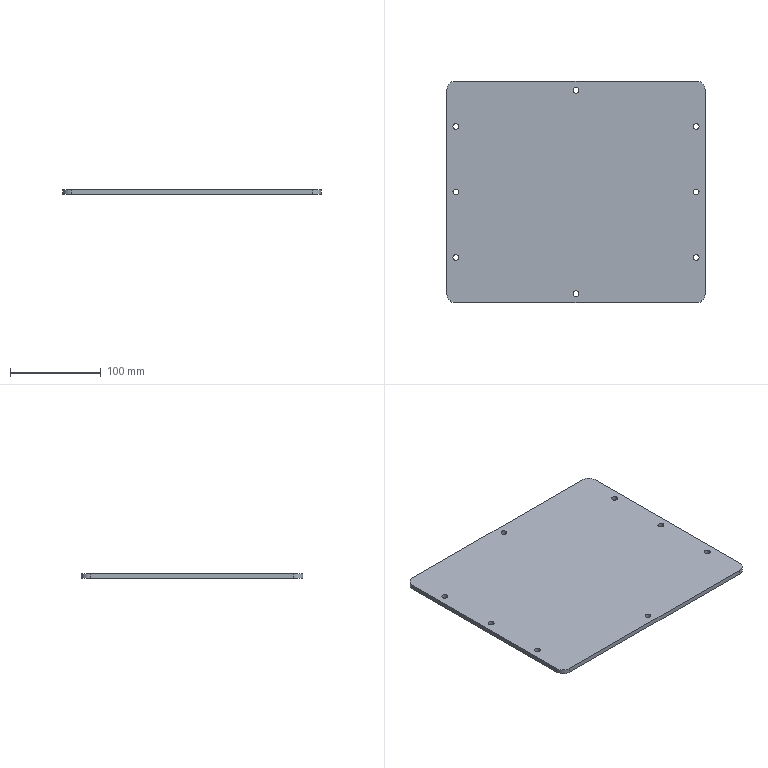Part | STEP file | 1 solid | 26 faces | box 284 x 244 x 5 mm | volume 344723 mm3 | cylinder 20 | plane 6 | commonest cylinder face diameters 6.5 x16 20 x4